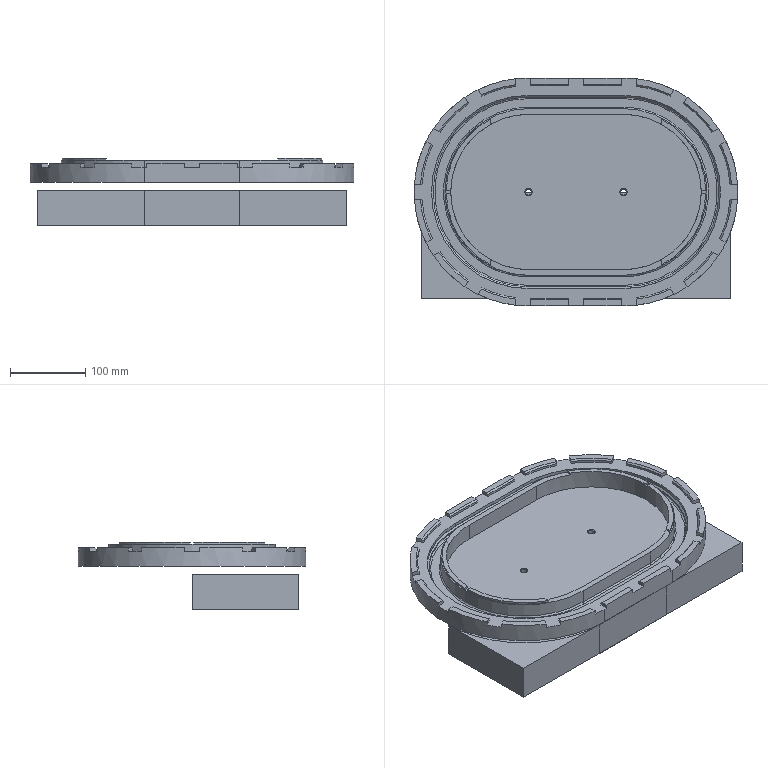NC program | NX | posted with a generic post | part box 429 x 302 x 89.371 mm
Lines 50401 to 52468 of 53366:
(PLANAR_MILL_2 , TOOL : D16开粗)
N100768 T02 M6
N100770 G53
N100772 G17 G0 G90 X220.4 Y-80.6 S6500 M3
N100774 G43 Z50. H2
N100776 Z1.5
N100778 G94 G1 Z-1.5 F3500.
N100780 X204.4
N100782 X189.25
N100784 G2 X179.05 Y-70.408 R10.2
N100786 G3 X63. Y45.55 R116.05
N100788 G1 X-63.
N100790 G3 X-179.05 Y-70.408 R116.05
N100792 G2 X-189.25 Y-80.6 R10.2
N100794 G1 X-204.4
N100796 X-220.4
N100798 Z1.5
N100800 G0 Z50.
N100802 X220.4
N100804 Z0.
N100806 G1 Z-3.
N100808 X204.4
N100810 X189.25
N100812 G2 X179.05 Y-70.408 R10.2
N100814 G3 X63. Y45.55 R116.05
N100816 G1 X-63.
N100818 G3 X-179.05 Y-70.408 R116.05
N100820 G2 X-189.25 Y-80.6 R10.2
N100822 G1 X-204.4
N100824 X-220.4
N100826 Z0.
N100828 G0 Z50.
N100830 X220.4
N100832 Z-1.5
N100834 G1 Z-4.5
N100836 X204.4
N100838 X189.25
N100840 G2 X179.05 Y-70.408 R10.2
N100842 G3 X63. Y45.55 R116.05
N100844 G1 X-63.
N100846 G3 X-179.05 Y-70.408 R116.05
N100848 G2 X-189.25 Y-80.6 R10.2
N100850 G1 X-204.4
N100852 X-220.4
N100854 Z-1.5
N100856 G0 Z50.
N100858 X220.4
N100860 Z-3.
N100862 G1 Z-6.
N100864 X204.4
N100866 X189.25
N100868 G2 X179.05 Y-70.408 R10.2
N100870 G3 X63. Y45.55 R116.05
N100872 G1 X-63.
N100874 G3 X-179.05 Y-70.408 R116.05
N100876 G2 X-189.25 Y-80.6 R10.2
N100878 G1 X-204.4
N100880 X-220.4
N100882 Z-3.
N100884 G0 Z50.
N100886 X220.4
N100888 Z-4.5
N100890 G1 Z-7.5
N100892 X204.4
N100894 X189.25
N100896 G2 X179.05 Y-70.408 R10.2
N100898 G3 X63. Y45.55 R116.05
N100900 G1 X-63.
N100902 G3 X-179.05 Y-70.408 R116.05
N100904 G2 X-189.25 Y-80.6 R10.2
N100906 G1 X-204.4
N100908 X-220.4
N100910 Z-4.5
N100912 G0 Z50.
N100914 X220.4
N100916 Z-6.
N100918 G1 Z-9.
N100920 X204.4
N100922 X189.25
N100924 G2 X179.05 Y-70.408 R10.2
N100926 G3 X63. Y45.55 R116.05
N100928 G1 X-63.
N100930 G3 X-179.05 Y-70.408 R116.05
N100932 G2 X-189.25 Y-80.6 R10.2
N100934 G1 X-204.4
N100936 X-220.4
N100938 Z-6.
N100940 G0 Z50.
N100942 X220.4
N100944 Z-7.5
N100946 G1 Z-10.5
N100948 X204.4
N100950 X189.25
N100952 G2 X179.05 Y-70.408 R10.2
N100954 G3 X63. Y45.55 R116.05
N100956 G1 X-63.
N100958 G3 X-179.05 Y-70.408 R116.05
N100960 G2 X-189.25 Y-80.6 R10.2
N100962 G1 X-204.4
N100964 X-220.4
N100966 Z-7.5
N100968 G0 Z50.
N100970 X220.4
N100972 Z-9.
N100974 G1 Z-12.
N100976 X204.4
N100978 X189.25
N100980 G2 X179.05 Y-70.408 R10.2
N100982 G3 X63. Y45.55 R116.05
N100984 G1 X-63.
N100986 G3 X-179.05 Y-70.408 R116.05
N100988 G2 X-189.25 Y-80.6 R10.2
N100990 G1 X-204.4
N100992 X-220.4
N100994 Z-9.
N100996 G0 Z50.
N100998 X220.4
N101000 Z-10.5
N101002 G1 Z-13.5
N101004 X204.4
N101006 X189.25
N101008 G2 X179.05 Y-70.408 R10.2
N101010 G3 X63. Y45.55 R116.05
N101012 G1 X-63.
N101014 G3 X-179.05 Y-70.408 R116.05
N101016 G2 X-189.25 Y-80.6 R10.2
N101018 G1 X-204.4
N101020 X-220.4
N101022 Z-10.5
N101024 G0 Z50.
N101026 X220.4
N101028 Z-12.
N101030 G1 Z-15.
N101032 X204.4
N101034 X189.25
N101036 G2 X179.05 Y-70.408 R10.2
N101038 G3 X63. Y45.55 R116.05
N101040 G1 X-63.
N101042 G3 X-179.05 Y-70.408 R116.05
N101044 G2 X-189.25 Y-80.6 R10.2
N101046 G1 X-204.4
N101048 X-220.4
N101050 Z-12.
N101052 G0 Z50.
N101054 X220.4
N101056 Z-13.5
N101058 G1 Z-16.5
N101060 X204.4
N101062 X189.25
N101064 G2 X179.05 Y-70.408 R10.2
N101066 G3 X63. Y45.55 R116.05
N101068 G1 X-63.
N101070 G3 X-179.05 Y-70.408 R116.05
N101072 G2 X-189.25 Y-80.6 R10.2
N101074 G1 X-204.4
N101076 X-220.4
N101078 Z-13.5
N101080 G0 Z50.
N101082 X220.4
N101084 Z-15.
N101086 G1 Z-18.
N101088 X204.4
N101090 X189.25
N101092 G2 X179.05 Y-70.408 R10.2
N101094 G3 X63. Y45.55 R116.05
N101096 G1 X-63.
N101098 G3 X-179.05 Y-70.408 R116.05
N101100 G2 X-189.25 Y-80.6 R10.2
N101102 G1 X-204.4
N101104 X-220.4
N101106 Z-15.
N101108 G0 Z50.
N101110 X220.4
N101112 Z-16.5
N101114 G1 Z-19.5
N101116 X204.4
N101118 X189.25
N101120 G2 X179.05 Y-70.408 R10.2
N101122 G3 X63. Y45.55 R116.05
N101124 G1 X-63.
N101126 G3 X-179.05 Y-70.408 R116.05
N101128 G2 X-189.25 Y-80.6 R10.2
N101130 G1 X-204.4
N101132 X-220.4
N101134 Z-16.5
N101136 G0 Z50.
N101138 X220.4
N101140 Z-18.
N101142 G1 Z-21.
N101144 X204.4
N101146 X189.25
N101148 G2 X179.05 Y-70.408 R10.2
N101150 G3 X63. Y45.55 R116.05
N101152 G1 X-63.
N101154 G3 X-179.05 Y-70.408 R116.05
N101156 G2 X-189.25 Y-80.6 R10.2
N101158 G1 X-204.4
N101160 X-220.4
N101162 Z-18.
N101164 G0 Z50.
N101166 X220.4
N101168 Z-19.5
N101170 G1 Z-22.5
N101172 X204.4
N101174 X189.25
N101176 G2 X179.05 Y-70.408 R10.2
N101178 G3 X63. Y45.55 R116.05
N101180 G1 X-63.
N101182 G3 X-179.05 Y-70.408 R116.05
N101184 G2 X-189.25 Y-80.6 R10.2
N101186 G1 X-204.4
N101188 X-220.4
N101190 Z-19.5
N101192 G0 Z50.
N101194 X220.4
N101196 Z-21.
N101198 G1 Z-24.
N101200 X204.4
N101202 X189.25
N101204 G2 X179.05 Y-70.408 R10.2
N101206 G3 X63. Y45.55 R116.05
N101208 G1 X-63.
N101210 G3 X-179.05 Y-70.408 R116.05
N101212 G2 X-189.25 Y-80.6 R10.2
N101214 G1 X-204.4
N101216 X-220.4
N101218 Z-21.
N101220 G0 Z50.
N101222 X220.4
N101224 Z-22.5
N101226 G1 Z-25.5
N101228 X204.4
N101230 X189.25
N101232 G2 X179.05 Y-70.408 R10.2
N101234 G3 X63. Y45.55 R116.05
N101236 G1 X-63.
N101238 G3 X-179.05 Y-70.408 R116.05
N101240 G2 X-189.25 Y-80.6 R10.2
N101242 G1 X-204.4
N101244 X-220.4
N101246 Z-22.5
N101248 G0 Z50.
N101250 X220.4
N101252 Z-24.
N101254 G1 Z-27.
N101256 X204.4
N101258 X189.25
N101260 G2 X179.05 Y-70.408 R10.2
N101262 G3 X63. Y45.55 R116.05
N101264 G1 X-63.
N101266 G3 X-179.05 Y-70.408 R116.05
N101268 G2 X-189.25 Y-80.6 R10.2
N101270 G1 X-204.4
N101272 X-220.4
N101274 Z-24.
N101276 G0 Z50.
N101278 X220.4
N101280 Z-25.5
N101282 G1 Z-28.5
N101284 X204.4
N101286 X189.25
N101288 G2 X179.05 Y-70.408 R10.2
N101290 G3 X63. Y45.55 R116.05
N101292 G1 X-63.
N101294 G3 X-179.05 Y-70.408 R116.05
N101296 G2 X-189.25 Y-80.6 R10.2
N101298 G1 X-204.4
N101300 X-220.4
N101302 Z-25.5
N101304 G0 Z50.
N101306 X220.4
N101308 Z-27.
N101310 G1 Z-30.
N101312 X204.4
N101314 X189.25
N101316 G2 X179.05 Y-70.408 R10.2
N101318 G3 X63. Y45.55 R116.05
N101320 G1 X-63.
N101322 G3 X-179.05 Y-70.408 R116.05
N101324 G2 X-189.25 Y-80.6 R10.2
N101326 G1 X-204.4
N101328 X-220.4
N101330 Z-27.
N101332 G0 Z50.
N101334 X220.4
N101336 Z-28.5
N101338 G1 Z-31.5
N101340 X204.4
N101342 X189.25
N101344 G2 X179.05 Y-70.408 R10.2
N101346 G3 X63. Y45.55 R116.05
N101348 G1 X-63.
N101350 G3 X-179.05 Y-70.408 R116.05
N101352 G2 X-189.25 Y-80.6 R10.2
N101354 G1 X-204.4
N101356 X-220.4
N101358 Z-28.5
N101360 G0 Z50.
N101362 X220.4
N101364 Z-30.
N101366 G1 Z-33.
N101368 X204.4
N101370 X189.25
N101372 G2 X179.05 Y-70.408 R10.2
N101374 G3 X63. Y45.55 R116.05
N101376 G1 X-63.
N101378 G3 X-179.05 Y-70.408 R116.05
N101380 G2 X-189.25 Y-80.6 R10.2
N101382 G1 X-204.4
N101384 X-220.4
N101386 Z-30.
N101388 G0 Z50.
N101390 X220.4
N101392 Z-31.5
N101394 G1 Z-34.5
N101396 X204.4
N101398 X189.25
N101400 G2 X179.05 Y-70.408 R10.2
N101402 G3 X63. Y45.55 R116.05
N101404 G1 X-63.
N101406 G3 X-179.05 Y-70.408 R116.05
N101408 G2 X-189.25 Y-80.6 R10.2
N101410 G1 X-204.4
N101412 X-220.4
N101414 Z-31.5
N101416 G0 Z50.
N101418 X220.4
N101420 Z-33.
N101422 G1 Z-36.
N101424 X204.4
N101426 X189.25
N101428 G2 X179.05 Y-70.408 R10.2
N101430 G3 X63. Y45.55 R116.05
N101432 G1 X-63.
N101434 G3 X-179.05 Y-70.408 R116.05
N101436 G2 X-189.25 Y-80.6 R10.2
N101438 G1 X-204.4
N101440 X-220.4
N101442 Z-33.
N101444 G0 Z50.
N101446 X220.4
N101448 Z-34.5
N101450 G1 Z-37.5
N101452 X204.4
N101454 X189.25
N101456 G2 X179.05 Y-70.408 R10.2
N101458 G3 X63. Y45.55 R116.05
N101460 G1 X-63.
N101462 G3 X-179.05 Y-70.408 R116.05
N101464 G2 X-189.25 Y-80.6 R10.2
N101466 G1 X-204.4
N101468 X-220.4
N101470 Z-34.5
N101472 G0 Z50.
N101474 X220.4
N101476 Z-36.
N101478 G1 Z-39.
N101480 X204.4
N101482 X189.25
N101484 G2 X179.05 Y-70.408 R10.2
N101486 G3 X63. Y45.55 R116.05
N101488 G1 X-63.
N101490 G3 X-179.05 Y-70.408 R116.05
N101492 G2 X-189.25 Y-80.6 R10.2
N101494 G1 X-204.4
N101496 X-220.4
N101498 Z-36.
N101500 G0 Z50.
N101502 X220.4
N101504 Z-37.5
N101506 G1 Z-40.5
N101508 X204.4
N101510 X189.25
N101512 G2 X179.05 Y-70.408 R10.2
N101514 G3 X63. Y45.55 R116.05
N101516 G1 X-63.
N101518 G3 X-179.05 Y-70.408 R116.05
N101520 G2 X-189.25 Y-80.6 R10.2
N101522 G1 X-204.4
N101524 X-220.4
N101526 Z-37.5
N101528 G0 Z50.
N101530 X220.4
N101532 Z-39.
N101534 G1 Z-42.
N101536 X204.4
N101538 X189.25
N101540 G2 X179.05 Y-70.408 R10.2
N101542 G3 X63. Y45.55 R116.05
N101544 G1 X-63.
N101546 G3 X-179.05 Y-70.408 R116.05
N101548 G2 X-189.25 Y-80.6 R10.2
N101550 G1 X-204.4
N101552 X-220.4
N101554 Z-39.
N101556 G0 Z50.
N101558 X220.4
N101560 Z-40.5
N101562 G1 Z-43.5
N101564 X204.4
N101566 X189.25
N101568 G2 X179.05 Y-70.408 R10.2
N101570 G3 X63. Y45.55 R116.05
N101572 G1 X-63.
N101574 G3 X-179.05 Y-70.408 R116.05
N101576 G2 X-189.25 Y-80.6 R10.2
N101578 G1 X-204.4
N101580 X-220.4
N101582 Z-40.5
N101584 G0 Z50.
N101586 X220.4
N101588 Z-42.
N101590 G1 Z-45.
N101592 X204.4
N101594 X189.25
N101596 G2 X179.05 Y-70.408 R10.2
N101598 G3 X63. Y45.55 R116.05
N101600 G1 X-63.
N101602 G3 X-179.05 Y-70.408 R116.05
N101604 G2 X-189.25 Y-80.6 R10.2
N101606 G1 X-204.4
N101608 X-220.4
N101610 Z-42.
N101612 G0 Z50.
N101614 X220.4
N101616 Z-43.5
N101618 G1 Z-46.5
N101620 X204.4
N101622 X189.25
N101624 G2 X179.05 Y-70.408 R10.2
N101626 G3 X63. Y45.55 R116.05
N101628 G1 X-63.
N101630 G3 X-179.05 Y-70.408 R116.05
N101632 G2 X-189.25 Y-80.6 R10.2
N101634 G1 X-204.4
N101636 X-220.4
N101638 Z-43.5
N101640 G0 Z50.
N101642 X220.4
N101644 Z-45.
N101646 G1 Z-48.
N101648 X204.4
N101650 X189.25
N101652 G2 X179.05 Y-70.408 R10.2
N101654 G3 X63. Y45.55 R116.05
N101656 G1 X-63.
N101658 G3 X-179.05 Y-70.408 R116.05
N101660 G2 X-189.25 Y-80.6 R10.2
N101662 G1 X-204.4
N101664 X-220.4
N101666 Z-45.
N101668 G0 Z50.
N101670 X220.4
N101672 Z-46.5
N101674 G1 Z-49.5
N101676 X204.4
N101678 X189.25
N101680 G2 X179.05 Y-70.408 R10.2
N101682 G3 X63. Y45.55 R116.05
N101684 G1 X-63.
N101686 G3 X-179.05 Y-70.408 R116.05
N101688 G2 X-189.25 Y-80.6 R10.2
N101690 G1 X-204.4
N101692 X-220.4
N101694 Z-46.5
N101696 G0 Z50.
N101698 X220.4
N101700 Z-46.8
N101702 G1 Z-49.8
N101704 X204.4
N101706 X189.25
N101708 G2 X179.05 Y-70.408 R10.2
N101710 G3 X63. Y45.55 R116.05
N101712 G1 X-63.
N101714 G3 X-179.05 Y-70.408 R116.05
N101716 G2 X-189.25 Y-80.6 R10.2
N101718 G1 X-204.4
N101720 X-220.4
N101722 Z-46.8
N101724 G0 Z50.
(PLANAR_MILL_2_COPY_2 , TOOL : D16开粗)
N101726 X184.207 Y-79.408
N101728 Z2.
N101730 G1 Z-1. F3000.
N101732 X184.2 Y-70.408
N101734 G3 X63.5 Y50.2 R120.7
N101736 G1 X-63.5
N101738 G3 X-184.2 Y-70.408 R120.7
N101740 G1 X-184.207 Y-79.408
N101742 Z2.
N101744 G0 Z50.
N101746 X184.207
N101748 Z1.
N101750 G1 Z-2.
N101752 X184.2 Y-70.408
N101754 G3 X63.5 Y50.2 R120.7
N101756 G1 X-63.5
N101758 G3 X-184.2 Y-70.408 R120.7
N101760 G1 X-184.207 Y-79.408
N101762 Z1.
N101764 G0 Z50.
N101766 X184.207
N101768 Z0.
N101770 G1 Z-3.
N101772 X184.2 Y-70.408
N101774 G3 X63.5 Y50.2 R120.7
N101776 G1 X-63.5
N101778 G3 X-184.2 Y-70.408 R120.7
N101780 G1 X-184.207 Y-79.408
N101782 Z0.
N101784 G0 Z50.
N101786 X184.207
N101788 Z-1.
N101790 G1 Z-4.
N101792 X184.2 Y-70.408
N101794 G3 X63.5 Y50.2 R120.7
N101796 G1 X-63.5
N101798 G3 X-184.2 Y-70.408 R120.7
N101800 G1 X-184.207 Y-79.408
N101802 Z-1.
N101804 G0 Z50.
N101806 X184.207
N101808 Z-2.
N101810 G1 Z-5.
N101812 X184.2 Y-70.408
N101814 G3 X63.5 Y50.2 R120.7
N101816 G1 X-63.5
N101818 G3 X-184.2 Y-70.408 R120.7
N101820 G1 X-184.207 Y-79.408
N101822 Z-2.
N101824 G0 Z50.
N101826 X184.207
N101828 Z-3.
N101830 G1 Z-6.
N101832 X184.2 Y-70.408
N101834 G3 X63.5 Y50.2 R120.7
N101836 G1 X-63.5
N101838 G3 X-184.2 Y-70.408 R120.7
N101840 G1 X-184.207 Y-79.408
N101842 Z-3.
N101844 G0 Z50.
N101846 X184.207
N101848 Z-4.
N101850 G1 Z-7.
N101852 X184.2 Y-70.408
N101854 G3 X63.5 Y50.2 R120.7
N101856 G1 X-63.5
N101858 G3 X-184.2 Y-70.408 R120.7
N101860 G1 X-184.207 Y-79.408
N101862 Z-4.
N101864 G0 Z50.
N101866 X184.207
N101868 Z-5.
N101870 G1 Z-8.
N101872 X184.2 Y-70.408
N101874 G3 X63.5 Y50.2 R120.7
N101876 G1 X-63.5
N101878 G3 X-184.2 Y-70.408 R120.7
N101880 G1 X-184.207 Y-79.408
N101882 Z-5.
N101884 G0 Z50.
N101886 X184.207
N101888 Z-6.
N101890 G1 Z-9.
N101892 X184.2 Y-70.408
N101894 G3 X63.5 Y50.2 R120.7
N101896 G1 X-63.5
N101898 G3 X-184.2 Y-70.408 R120.7
N101900 G1 X-184.207 Y-79.408
N101902 Z-6.
N101904 G0 Z50.
N101906 X184.207
N101908 Z-7.
N101910 G1 Z-10.
N101912 X184.2 Y-70.408
N101914 G3 X63.5 Y50.2 R120.7
N101916 G1 X-63.5
N101918 G3 X-184.2 Y-70.408 R120.7
N101920 G1 X-184.207 Y-79.408
N101922 Z-7.
N101924 G0 Z50.
N101926 X184.207
N101928 Z-8.
N101930 G1 Z-11.
N101932 X184.2 Y-70.408
N101934 G3 X63.5 Y50.2 R120.7
N101936 G1 X-63.5
N101938 G3 X-184.2 Y-70.408 R120.7
N101940 G1 X-184.207 Y-79.408
N101942 Z-8.
N101944 G0 Z50.
N101946 X184.207
N101948 Z-9.
N101950 G1 Z-12.
N101952 X184.2 Y-70.408
N101954 G3 X63.5 Y50.2 R120.7
N101956 G1 X-63.5
N101958 G3 X-184.2 Y-70.408 R120.7
N101960 G1 X-184.207 Y-79.408
N101962 Z-9.
N101964 G0 Z50.
N101966 X184.207
N101968 Z-10.
N101970 G1 Z-13.
N101972 X184.2 Y-70.408
N101974 G3 X63.5 Y50.2 R120.7
N101976 G1 X-63.5
N101978 G3 X-184.2 Y-70.408 R120.7
N101980 G1 X-184.207 Y-79.408
N101982 Z-10.
N101984 G0 Z50.
N101986 X184.207
N101988 Z-11.
N101990 G1 Z-14.
N101992 X184.2 Y-70.408
N101994 G3 X63.5 Y50.2 R120.7
N101996 G1 X-63.5
N101998 G3 X-184.2 Y-70.408 R120.7
N102000 G1 X-184.207 Y-79.408
N102002 Z-11.
N102004 G0 Z50.
N102006 X184.207
N102008 Z-12.
N102010 G1 Z-15.
N102012 X184.2 Y-70.408
N102014 G3 X63.5 Y50.2 R120.7
N102016 G1 X-63.5
N102018 G3 X-184.2 Y-70.408 R120.7
N102020 G1 X-184.207 Y-79.408
N102022 Z-12.
N102024 G0 Z50.
N102026 X184.207
N102028 Z-13.
N102030 G1 Z-16.
N102032 X184.2 Y-70.408
N102034 G3 X63.5 Y50.2 R120.7
N102036 G1 X-63.5
N102038 G3 X-184.2 Y-70.408 R120.7
N102040 G1 X-184.207 Y-79.408
N102042 Z-13.
N102044 G0 Z50.
N102046 X184.207
N102048 Z-14.
N102050 G1 Z-17.
N102052 X184.2 Y-70.408
N102054 G3 X63.5 Y50.2 R120.7
N102056 G1 X-63.5
N102058 G3 X-184.2 Y-70.408 R120.7
N102060 G1 X-184.207 Y-79.408
N102062 Z-14.
N102064 G0 Z50.
N102066 X184.207
N102068 Z-15.
N102070 G1 Z-18.
N102072 X184.2 Y-70.408
N102074 G3 X63.5 Y50.2 R120.7
N102076 G1 X-63.5
N102078 G3 X-184.2 Y-70.408 R120.7
N102080 G1 X-184.207 Y-79.408
N102082 Z-15.
N102084 G0 Z50.
N102086 X184.207
N102088 Z-16.
N102090 G1 Z-19.
N102092 X184.2 Y-70.408
N102094 G3 X63.5 Y50.2 R120.7
N102096 G1 X-63.5
N102098 G3 X-184.2 Y-70.408 R120.7
N102100 G1 X-184.207 Y-79.408
N102102 Z-16.
N102104 G0 Z50.
N102106 X184.207
N102108 Z-17.
N102110 G1 Z-20.
N102112 X184.2 Y-70.408
N102114 G3 X63.5 Y50.2 R120.7
N102116 G1 X-63.5
N102118 G3 X-184.2 Y-70.408 R120.7
N102120 G1 X-184.207 Y-79.408
N102122 Z-17.
N102124 G0 Z50.
N102126 X184.207
N102128 Z-18.
N102130 G1 Z-21.
N102132 X184.2 Y-70.408
N102134 G3 X63.5 Y50.2 R120.7
N102136 G1 X-63.5
N102138 G3 X-184.2 Y-70.408 R120.7
N102140 G1 X-184.207 Y-79.408
N102142 Z-18.
N102144 G0 Z50.
N102146 X184.207
N102148 Z-19.
N102150 G1 Z-22.
N102152 X184.2 Y-70.408
N102154 G3 X63.5 Y50.2 R120.7
N102156 G1 X-63.5
N102158 G3 X-184.2 Y-70.408 R120.7
N102160 G1 X-184.207 Y-79.408
N102162 Z-19.
N102164 G0 Z50.
N102166 X184.207
N102168 Z-20.
N102170 G1 Z-23.
N102172 X184.2 Y-70.408
N102174 G3 X63.5 Y50.2 R120.7
N102176 G1 X-63.5
N102178 G3 X-184.2 Y-70.408 R120.7
N102180 G1 X-184.207 Y-79.408
N102182 Z-20.
N102184 G0 Z50.
N102186 X184.207
N102188 Z-20.886
N102190 G1 Z-23.886
N102192 X184.2 Y-70.408
N102194 G3 X63.5 Y50.2 R120.7
N102196 G1 X-63.5
N102198 G3 X-184.2 Y-70.408 R120.7
N102200 G1 X-184.207 Y-79.408
N102202 Z-20.886
N102204 G0 Z50.
(PLANAR_MILL_2_COPY_2_COPY , TOOL : D16开粗)
N102206 X184.312 Y-86.408
N102208 Z-20.886
N102210 G1 Z-23.886 F800.
N102212 X184.3 Y-70.408
N102214 G3 X63.5 Y50.3 R120.8
N102216 G1 X-63.5
N102218 G3 X-184.3 Y-70.408 R120.8
N102220 G1 X-184.312 Y-86.408
N102222 Z-20.886
N102224 G0 Z50.
(PLANAR_MILL_2_COPY_1 , TOOL : D16开粗)
N102226 X220.4 Y-80.5
N102228 Z-46.95
N102230 G1 Z-49.95
N102232 X204.4
N102234 X189.25
N102236 G2 X179.15 Y-70.408 R10.1
N102238 G3 X63. Y45.65 R116.15
N102240 G1 X-63.
N102242 G3 X-179.15 Y-70.408 R116.15
N102244 G2 X-189.25 Y-80.5 R10.1
N102246 G1 X-204.4
N102248 X-220.4
N102250 Z-46.95
N102252 G0 Z50.
N102254 M5
(FLOOR_FACING , TOOL : D63.)
N102256 T01 M6
N102258 G54
N102260 G17 G0 G90 X160.741 Y104.9 S4500 M3
N102262 G43 Z50. H1
N102264 Z3.
N102266 G94 G1 Z0. F1500.
N102268 Y101.9
N102270 Y-101.9
N102272 Y-104.9
N102274 Z3.
N102276 G0 Z50.
N102278 X116.236 Y104.9
N102280 Z3.
N102282 G1 Z0.
N102284 Y101.9
N102286 Y-101.9
N102288 Y-104.9
N102290 Z3.
N102292 G0 Z50.
N102294 X71.731 Y104.9
N102296 Z3.
N102298 G1 Z0.
N102300 Y101.9
N102302 Y-101.9
N102304 Y-104.9
N102306 Z3.
N102308 G0 Z50.
N102310 X27.226 Y104.9
N102312 Z3.
N102314 G1 Z0.
N102316 Y101.9
N102318 Y-101.9
N102320 Y-104.9
N102322 Z3.
N102324 G0 Z50.
N102326 X-17.279 Y104.9
N102328 Z3.
N102330 G1 Z0.
N102332 Y101.9
N102334 Y-101.9
N102336 Y-104.9
N102338 Z3.
N102340 G0 Z50.
N102342 X-61.784 Y104.9
N102344 Z3.
N102346 G1 Z0.
N102348 Y101.9
N102350 Y-101.9
N102352 Y-104.9
N102354 Z3.
N102356 G0 Z50.
N102358 X-106.289 Y104.9
N102360 Z3.
N102362 G1 Z0.
N102364 Y101.9
N102366 Y-101.9
N102368 Y-104.9
N102370 Z3.
N102372 G0 Z50.
N102374 X-150.794 Y127.755
N102376 Z3.
N102378 G1 Z0.
N102380 Y101.9
N102382 Y-101.9
N102384 Y-118.902
N102386 Z3.
N102388 G0 Z50.
N102390 M5
(DRILLING_COPY , TOOL : 倒角12.)
N102392 T03 M6
N102394 G54
N102396 G17 G0 G90 X-154.4 Y-30.4 S1500 M3
N102398 G43 Z50. H3
N102400 G94 G81 G98 Z-5.5 F150. R3.
N102402 X-74.4 Y29.6
N102404 X74.4
N102406 X154.4 Y-30.4
N102408 G80
N102410 G0 X154.4 Y-30.4 Z50.
N102412 M5
(DRILLING , TOOL : 钻头10.5)
N102414 T04 M6
N102416 G54
N102418 G17 G0 G90 X-154.4 Y-30.4 S1200 M3
N102420 G43 Z50. H4
N102422 G94 G83 G98 Z-57. F180. Q5. R3.
N102424 X-74.4 Y29.6
N102426 X74.4
N102428 X154.4 Y-30.4
N102430 G80
N102432 G0 X154.4 Y-30.4 Z50.
N102434 M5
(DRILLING_COPY_1 , TOOL : D16开粗)
N102436 T02 M6
N102438 G54
N102440 G17 G0 G90 X-154.4 Y-30.4 S700 M3
N102442 G43 Z50. H2
N102444 G94 G83 G98 Z-15. F120. Q2. R3.
N102446 X-74.4 Y29.6
N102448 X74.4
N102450 X154.4 Y-30.4
N102452 G80
N102454 G0 X154.4 Y-30.4 Z50.
N102456 M5
(PLANAR_MILL_COPY_1 , TOOL : D63.)
N102458 T01 M6
N102460 G54
N102462 G17 G0 G90 X-190.948 Y-63.003 S4500 M3
N102464 G43 Z50. H1
N102466 Z3.1
N102468 G94 G1 Z0.1 F1500.
N102470 X-190.9 Y-0.003
N102472 G2 X-63.5 Y127.3 R127.4
N102474 G1 X63.5
N102476 G2 X190.9 Y-0.003 R127.4
N102478 G1 X190.948 Y-63.003
N102480 Z3.1
N102482 G0 Z50.
N102484 M5
(PLANAR_MILL_2_COPY_2_COPY_1 , TOOL : D16开粗)
N102486 T02 M6
N102488 G54
N102490 G17 G0 G90 X213.4 Y-8.1 S6500 M3
N102492 G43 Z50. H2
N102494 Z1.5
N102496 G94 G1 Z-1.5 F3000.
N102498 X204.4
N102500 X194.4
N102502 G2 X186.3 Y-0.006 R8.1
N102504 G3 X63.5 Y122.7 R122.8
N102506 G1 X-63.5
N102508 G3 X-186.3 Y-0.006 R122.8
N102510 G2 X-194.4 Y-8.1 R8.1
N102512 G1 X-204.4
N102514 X-213.4
N102516 Z1.5
N102518 G0 Z3.
N102520 X213.4
N102522 Z0.
N102524 G1 Z-3.
N102526 X204.4
N102528 X194.4
N102530 G2 X186.3 Y-0.006 R8.1
N102532 G3 X63.5 Y122.7 R122.8
N102534 G1 X-63.5
N102536 G3 X-186.3 Y-0.006 R122.8
N102538 G2 X-194.4 Y-8.1 R8.1
N102540 G1 X-204.4
N102542 X-213.4
N102544 Z0.
N102546 G0 Z3.
N102548 X213.4
N102550 Z-1.5
N102552 G1 Z-4.5
N102554 X204.4
N102556 X194.4
N102558 G2 X186.3 Y-0.006 R8.1
N102560 G3 X63.5 Y122.7 R122.8
N102562 G1 X-63.5
N102564 G3 X-186.3 Y-0.006 R122.8
N102566 G2 X-194.4 Y-8.1 R8.1
N102568 G1 X-204.4
N102570 X-213.4
N102572 Z-1.5
N102574 G0 Z3.
N102576 X213.4
N102578 Z-3.
N102580 G1 Z-6.
N102582 X204.4
N102584 X194.4
N102586 G2 X186.3 Y-0.006 R8.1
N102588 G3 X63.5 Y122.7 R122.8
N102590 G1 X-63.5
N102592 G3 X-186.3 Y-0.006 R122.8
N102594 G2 X-194.4 Y-8.1 R8.1
N102596 G1 X-204.4
N102598 X-213.4
N102600 Z-3.
N102602 G0 Z3.
N102604 X213.4
N102606 Z-4.5
N102608 G1 Z-7.5
N102610 X204.4
N102612 X194.4
N102614 G2 X186.3 Y-0.006 R8.1
N102616 G3 X63.5 Y122.7 R122.8
N102618 G1 X-63.5
N102620 G3 X-186.3 Y-0.006 R122.8
N102622 G2 X-194.4 Y-8.1 R8.1
N102624 G1 X-204.4
N102626 X-213.4
N102628 Z-4.5
N102630 G0 Z3.
N102632 X213.4
N102634 Z-6.
N102636 G1 Z-9.
N102638 X204.4
N102640 X194.4
N102642 G2 X186.3 Y-0.006 R8.1
N102644 G3 X63.5 Y122.7 R122.8
N102646 G1 X-63.5
N102648 G3 X-186.3 Y-0.006 R122.8
N102650 G2 X-194.4 Y-8.1 R8.1
N102652 G1 X-204.4
N102654 X-213.4
N102656 Z-6.
N102658 G0 Z3.
N102660 X213.4
N102662 Z-7.5
N102664 G1 Z-10.5
N102666 X204.4
N102668 X194.4
N102670 G2 X186.3 Y-0.006 R8.1
N102672 G3 X63.5 Y122.7 R122.8
N102674 G1 X-63.5
N102676 G3 X-186.3 Y-0.006 R122.8
N102678 G2 X-194.4 Y-8.1 R8.1
N102680 G1 X-204.4
N102682 X-213.4
N102684 Z-7.5
N102686 G0 Z3.
N102688 X213.4
N102690 Z-9.
N102692 G1 Z-12.
N102694 X204.4
N102696 X194.4
N102698 G2 X186.3 Y-0.006 R8.1
N102700 G3 X63.5 Y122.7 R122.8
N102702 G1 X-63.5
N102704 G3 X-186.3 Y-0.006 R122.8
N102706 G2 X-194.4 Y-8.1 R8.1
N102708 G1 X-204.4
N102710 X-213.4
N102712 Z-9.
N102714 G0 Z3.
N102716 X213.4
N102718 Z-10.5
N102720 G1 Z-13.5
N102722 X204.4
N102724 X194.4
N102726 G2 X186.3 Y-0.006 R8.1
N102728 G3 X63.5 Y122.7 R122.8
N102730 G1 X-63.5
N102732 G3 X-186.3 Y-0.006 R122.8
N102734 G2 X-194.4 Y-8.1 R8.1
N102736 G1 X-204.4
N102738 X-213.4
N102740 Z-10.5
N102742 G0 Z3.
N102744 X213.4
N102746 Z-12.
N102748 G1 Z-15.
N102750 X204.4
N102752 X194.4
N102754 G2 X186.3 Y-0.006 R8.1
N102756 G3 X63.5 Y122.7 R122.8
N102758 G1 X-63.5
N102760 G3 X-186.3 Y-0.006 R122.8
N102762 G2 X-194.4 Y-8.1 R8.1
N102764 G1 X-204.4
N102766 X-213.4
N102768 Z-12.
N102770 G0 Z3.
N102772 X213.4
N102774 Z-13.5
N102776 G1 Z-16.5
N102778 X204.4
N102780 X194.4
N102782 G2 X186.3 Y-0.006 R8.1
N102784 G3 X63.5 Y122.7 R122.8
N102786 G1 X-63.5
N102788 G3 X-186.3 Y-0.006 R122.8
N102790 G2 X-194.4 Y-8.1 R8.1
N102792 G1 X-204.4
N102794 X-213.4
N102796 Z-13.5
N102798 G0 Z3.
N102800 X213.4
N102802 Z-15.
N102804 G1 Z-18.
N102806 X204.4
N102808 X194.4
N102810 G2 X186.3 Y-0.006 R8.1
N102812 G3 X63.5 Y122.7 R122.8
N102814 G1 X-63.5
N102816 G3 X-186.3 Y-0.006 R122.8
N102818 G2 X-194.4 Y-8.1 R8.1
N102820 G1 X-204.4
N102822 X-213.4
N102824 Z-15.
N102826 G0 Z3.
N102828 X213.4
N102830 Z-16.5
N102832 G1 Z-19.5
N102834 X204.4
N102836 X194.4
N102838 G2 X186.3 Y-0.006 R8.1
N102840 G3 X63.5 Y122.7 R122.8
N102842 G1 X-63.5
N102844 G3 X-186.3 Y-0.006 R122.8
N102846 G2 X-194.4 Y-8.1 R8.1
N102848 G1 X-204.4
N102850 X-213.4
N102852 Z-16.5
N102854 G0 Z3.
N102856 X213.4
N102858 Z-18.
N102860 G1 Z-21.
N102862 X204.4
N102864 X194.4
N102866 G2 X186.3 Y-0.006 R8.1
N102868 G3 X63.5 Y122.7 R122.8
N102870 G1 X-63.5
N102872 G3 X-186.3 Y-0.006 R122.8
N102874 G2 X-194.4 Y-8.1 R8.1
N102876 G1 X-204.4
N102878 X-213.4
N102880 Z-18.
N102882 G0 Z3.
N102884 X213.4
N102886 Z-19.5
N102888 G1 Z-22.5
N102890 X204.4
N102892 X194.4
N102894 G2 X186.3 Y-0.006 R8.1
N102896 G3 X63.5 Y122.7 R122.8
N102898 G1 X-63.5
N102900 G3 X-186.3 Y-0.006 R122.8
N102902 G2 X-194.4 Y-8.1 R8.1
N102904 G1 X-204.4
N102906 X-213.4
N102908 Z-19.5
N102910 G0 Z3.
N102912 X213.4
N102914 Z-21.
N102916 G1 Z-24.
N102918 X204.4
N102920 X194.4
N102922 G2 X186.3 Y-0.006 R8.1
N102924 G3 X63.5 Y122.7 R122.8
N102926 G1 X-63.5
N102928 G3 X-186.3 Y-0.006 R122.8
N102930 G2 X-194.4 Y-8.1 R8.1
N102932 G1 X-204.4
N102934 X-213.4
N102936 Z-21.
N102938 G0 Z3.
N102940 X213.4
N102942 Z-22.5
N102944 G1 Z-25.5
N102946 X204.4
N102948 X194.4
N102950 G2 X186.3 Y-0.006 R8.1
N102952 G3 X63.5 Y122.7 R122.8
N102954 G1 X-63.5
N102956 G3 X-186.3 Y-0.006 R122.8
N102958 G2 X-194.4 Y-8.1 R8.1
N102960 G1 X-204.4
N102962 X-213.4
N102964 Z-22.5
N102966 G0 Z3.
N102968 X213.4
N102970 Z-22.786
N102972 G1 Z-25.786
N102974 X204.4
N102976 X194.4
N102978 G2 X186.3 Y-0.006 R8.1
N102980 G3 X63.5 Y122.7 R122.8
N102982 G1 X-63.5
N102984 G3 X-186.3 Y-0.006 R122.8
N102986 G2 X-194.4 Y-8.1 R8.1
N102988 G1 X-204.4
N102990 X-213.4
N102992 Z-22.786
N102994 G0 Z50.
(PLANAR_MILL_2_COPY_3 , TOOL : D16开粗)
N102996 X220.4
N102998 Z-21.886
N103000 G1 Z-24.886 F3500.
N103002 X204.4
N103004 X189.25
N103006 G2 X181.15 Y-0.006 R8.1
N103008 G3 X63. Y118.05 R118.15
N103010 G1 X-63.
N103012 G3 X-181.15 Y-0.006 R118.15
N103014 G2 X-189.25 Y-8.1 R8.1
N103016 G1 X-204.4
N103018 X-220.4
N103020 Z-21.886
N103022 G0 Z50.
N103024 X220.4
N103026 Z-23.386
N103028 G1 Z-26.386
N103030 X204.4
N103032 X189.25
N103034 G2 X181.15 Y-0.006 R8.1
N103036 G3 X63. Y118.05 R118.15
N103038 G1 X-63.
N103040 G3 X-181.15 Y-0.006 R118.15
N103042 G2 X-189.25 Y-8.1 R8.1
N103044 G1 X-204.4
N103046 X-220.4
N103048 Z-23.386
N103050 G0 Z50.
N103052 X220.4
N103054 Z-24.886
N103056 G1 Z-27.886
N103058 X204.4
N103060 X189.25
N103062 G2 X181.15 Y-0.006 R8.1
N103064 G3 X63. Y118.05 R118.15
N103066 G1 X-63.
N103068 G3 X-181.15 Y-0.006 R118.15
N103070 G2 X-189.25 Y-8.1 R8.1
N103072 G1 X-204.4
N103074 X-220.4
N103076 Z-24.886
N103078 G0 Z50.
N103080 X220.4
N103082 Z-26.386
N103084 G1 Z-29.386
N103086 X204.4
N103088 X189.25
N103090 G2 X181.15 Y-0.006 R8.1
N103092 G3 X63. Y118.05 R118.15
N103094 G1 X-63.
N103096 G3 X-181.15 Y-0.006 R118.15
N103098 G2 X-189.25 Y-8.1 R8.1
N103100 G1 X-204.4
N103102 X-220.4
N103104 Z-26.386
N103106 G0 Z50.
N103108 X220.4
N103110 Z-27.886
N103112 G1 Z-30.886
N103114 X204.4
N103116 X189.25
N103118 G2 X181.15 Y-0.006 R8.1
N103120 G3 X63. Y118.05 R118.15
N103122 G1 X-63.
N103124 G3 X-181.15 Y-0.006 R118.15
N103126 G2 X-189.25 Y-8.1 R8.1
N103128 G1 X-204.4
N103130 X-220.4
N103132 Z-27.886
N103134 G0 Z50.
N103136 X220.4
N103138 Z-29.386
N103140 G1 Z-32.386
N103142 X204.4
N103144 X189.25
N103146 G2 X181.15 Y-0.006 R8.1
N103148 G3 X63. Y118.05 R118.15
N103150 G1 X-63.
N103152 G3 X-181.15 Y-0.006 R118.15
N103154 G2 X-189.25 Y-8.1 R8.1
N103156 G1 X-204.4
N103158 X-220.4
N103160 Z-29.386
N103162 G0 Z50.
N103164 X220.4
N103166 Z-30.886
N103168 G1 Z-33.886
N103170 X204.4
N103172 X189.25
N103174 G2 X181.15 Y-0.006 R8.1
N103176 G3 X63. Y118.05 R118.15
N103178 G1 X-63.
N103180 G3 X-181.15 Y-0.006 R118.15
N103182 G2 X-189.25 Y-8.1 R8.1
N103184 G1 X-204.4
N103186 X-220.4
N103188 Z-30.886
N103190 G0 Z50.
N103192 X220.4
N103194 Z-32.386
N103196 G1 Z-35.386
N103198 X204.4
N103200 X189.25
N103202 G2 X181.15 Y-0.006 R8.1
N103204 G3 X63. Y118.05 R118.15
N103206 G1 X-63.
N103208 G3 X-181.15 Y-0.006 R118.15
N103210 G2 X-189.25 Y-8.1 R8.1
N103212 G1 X-204.4
N103214 X-220.4
N103216 Z-32.386
N103218 G0 Z50.
N103220 X220.4
N103222 Z-33.886
N103224 G1 Z-36.886
N103226 X204.4
N103228 X189.25
N103230 G2 X181.15 Y-0.006 R8.1
N103232 G3 X63. Y118.05 R118.15
N103234 G1 X-63.
N103236 G3 X-181.15 Y-0.006 R118.15
N103238 G2 X-189.25 Y-8.1 R8.1
N103240 G1 X-204.4
N103242 X-220.4
N103244 Z-33.886
N103246 G0 Z50.
N103248 X220.4
N103250 Z-35.386
N103252 G1 Z-38.386
N103254 X204.4
N103256 X189.25
N103258 G2 X181.15 Y-0.006 R8.1
N103260 G3 X63. Y118.05 R118.15
N103262 G1 X-63.
N103264 G3 X-181.15 Y-0.006 R118.15
N103266 G2 X-189.25 Y-8.1 R8.1
N103268 G1 X-204.4
N103270 X-220.4
N103272 Z-35.386
N103274 G0 Z50.
N103276 X220.4
N103278 Z-36.886
N103280 G1 Z-39.886
N103282 X204.4
N103284 X189.25
N103286 G2 X181.15 Y-0.006 R8.1
N103288 G3 X63. Y118.05 R118.15
N103290 G1 X-63.
N103292 G3 X-181.15 Y-0.006 R118.15
N103294 G2 X-189.25 Y-8.1 R8.1
N103296 G1 X-204.4
N103298 X-220.4
N103300 Z-36.886
N103302 G0 Z50.
N103304 X220.4
N103306 Z-38.386
N103308 G1 Z-41.386
N103310 X204.4
N103312 X189.25
N103314 G2 X181.15 Y-0.006 R8.1
N103316 G3 X63. Y118.05 R118.15
N103318 G1 X-63.
N103320 G3 X-181.15 Y-0.006 R118.15
N103322 G2 X-189.25 Y-8.1 R8.1
N103324 G1 X-204.4
N103326 X-220.4
N103328 Z-38.386
N103330 G0 Z50.
N103332 X220.4
N103334 Z-39.886
N103336 G1 Z-42.886
N103338 X204.4
N103340 X189.25
N103342 G2 X181.15 Y-0.006 R8.1
N103344 G3 X63. Y118.05 R118.15
N103346 G1 X-63.
N103348 G3 X-181.15 Y-0.006 R118.15
N103350 G2 X-189.25 Y-8.1 R8.1
N103352 G1 X-204.4
N103354 X-220.4
N103356 Z-39.886
N103358 G0 Z50.
N103360 X220.4
N103362 Z-41.386
N103364 G1 Z-44.386
N103366 X204.4
N103368 X189.25
N103370 G2 X181.15 Y-0.006 R8.1
N103372 G3 X63. Y118.05 R118.15
N103374 G1 X-63.
N103376 G3 X-181.15 Y-0.006 R118.15
N103378 G2 X-189.25 Y-8.1 R8.1
N103380 G1 X-204.4
N103382 X-220.4
N103384 Z-41.386
N103386 G0 Z50.
N103388 X220.4
N103390 Z-42.886
N103392 G1 Z-45.886
N103394 X204.4
N103396 X189.25
N103398 G2 X181.15 Y-0.006 R8.1
N103400 G3 X63. Y118.05 R118.15
N103402 G1 X-63.
N103404 G3 X-181.15 Y-0.006 R118.15
N103406 G2 X-189.25 Y-8.1 R8.1
N103408 G1 X-204.4
N103410 X-220.4
N103412 Z-42.886
N103414 G0 Z50.
N103416 X220.4
N103418 Z-44.
N103420 G1 Z-47.
N103422 X204.4
N103424 X189.25
N103426 G2 X181.15 Y-0.006 R8.1
N103428 G3 X63. Y118.05 R118.15
N103430 G1 X-63.
N103432 G3 X-181.15 Y-0.006 R118.15
N103434 G2 X-189.25 Y-8.1 R8.1
N103436 G1 X-204.4
N103438 X-220.4
N103440 Z-44.
N103442 G0 Z50.
(CURVE_DRIVE , TOOL : D16开粗)
N103444 X182.975 Y-3.006 S5000
N103446 Z-20.4
N103448 G1 Z-22.785 F3000.
N103450 X182.974 Y-2.904 Z-23.562
N103452 X182.971 Y-2.604 Z-24.285
N103454 X182.967 Y-2.128 Z-24.907
N103456 X182.962 Y-1.506 Z-25.383
N103458 X182.955 Y-0.783 Z-25.683
N103460 X182.948 Y-0.006 Z-25.785
N103462 G3 X61.954 Y119.848 R119.956
N103464 G1 X57.823
N103466 X49.563
N103468 X33.042
N103470 X0.
N103472 X-33.042
N103474 X-49.563
N103476 X-57.823
N103478 X-61.954
N103480 G3 X-182.931 Y1.937 R119.956
N103482 G1 X-182.948 Y-0.006
N103484 X-182.788 Y-0.007 Z-25.992
N103486 X-182.594 Z-26.188
N103488 G2 X-61.894 Y119.495 R119.603
N103490 G1 X-57.768
N103492 X-49.515
N103494 X-33.01
N103496 X0.
N103498 X33.01
N103500 X49.515
N103502 X57.768
N103504 X61.894
N103506 G2 X182.577 Y1.919 R119.603
N103508 G1 X182.594 Y-0.007
N103510 X182.399 Z-26.384
N103512 X182.325 Z-26.489
N103514 X182.29 Z-26.609
N103516 G3 X61.835 Y119.19 R119.3
N103518 G1 X57.712
N103520 X49.468
N103522 X32.978
N103524 X0.
N103526 X-32.978
N103528 X-49.468
N103530 X-57.712
N103532 X-61.835
N103534 G3 X-182.273 Y1.929 R119.3
N103536 G1 X-182.29 Y-0.007
N103538 X-182.161 Z-27.089
N103540 G2 X-61.775 Y119.061 R119.172
N103542 G1 X-57.657
N103544 X-49.42
N103546 X-32.947
N103548 X0.
N103550 X32.947
N103552 X49.42
N103554 X57.657
N103556 X61.775
N103558 G2 X182.144 Y1.913 R119.172
N103560 G1 X182.161 Y-0.007
N103562 X182.033 Z-27.57
N103564 G3 X61.715 Y118.933 R119.044
N103566 G1 X57.601
N103568 X49.372
N103570 X32.915
N103572 X0.
N103574 X-32.915
N103576 X-49.372
N103578 X-57.601
N103580 X-61.715
N103582 G3 X-182.015 Y1.928 R119.045
N103584 G1 X-182.033 Y-0.007
N103586 X-181.904 Z-28.051
N103588 G2 X-61.656 Y118.804 R118.917
N103590 G1 X-57.545
N103592 X-49.325
N103594 X-32.883
N103596 X0.
N103598 X32.883
N103600 X49.325
N103602 X57.545
N103604 X61.656
N103606 G2 X181.887 Y1.91 R118.917
N103608 G1 X181.904 Y-0.007
N103610 X181.775 Z-28.532
N103612 G3 X61.596 Y118.675 R118.789
N103614 G1 X57.49
N103616 X49.277
N103618 X32.851
N103620 X0.
N103622 X-32.851
N103624 X-49.277
N103626 X-57.49
N103628 X-61.596
N103630 G3 X-181.758 Y1.927 R118.789
N103632 G1 X-181.775 Y-0.007
N103634 X-181.646 Z-29.013
N103636 G2 X-61.537 Y118.546 R118.661
N103638 G1 X-57.434
N103640 X-49.229
N103642 X-32.82
N103644 X0.
N103646 X32.82
N103648 X49.229
N103650 X57.434
N103652 X61.537
N103654 G2 X181.629 Y1.907 R118.662
N103656 G1 X181.646 Y-0.007
N103658 X181.517 Z-29.493
N103660 G3 X61.477 Y118.417 R118.534
N103662 G1 X57.379
N103664 X49.182
N103666 X32.788
N103668 X0.
N103670 X-32.788
N103672 X-49.182
N103674 X-57.379
N103676 X-61.477
N103678 G3 X-181.5 Y1.926 R118.534
N103680 G1 X-181.517 Y-0.007
N103682 X-181.388 Z-29.974
N103684 G2 X-61.418 Y118.288 R118.406
N103686 G1 X-57.323
N103688 X-49.134
N103690 X-32.756
N103692 X0.
N103694 X32.756
N103696 X49.134
N103698 X57.323
N103700 X61.418
N103702 G2 X181.371 Y1.904 R118.407
N103704 G1 X181.388 Y-0.007
N103706 X181.26 Z-30.455
N103708 G3 X61.358 Y118.16 R118.279
N103710 G1 X57.267
N103712 X49.086
N103714 X32.724
N103716 X0.
N103718 X-32.724
N103720 X-49.086
N103722 X-57.267
N103724 X-61.358
N103726 G3 X-181.242 Y1.925 R118.279
N103728 G1 X-181.26 Y-0.007
N103730 X-181.131 Z-30.936
N103732 G2 X-61.298 Y118.031 R118.151
N103734 G1 X-57.212
N103736 X-49.039
N103738 X-32.693
N103740 X0.
N103742 X32.693
N103744 X49.039
N103746 X57.212
N103748 X61.298
N103750 G2 X181.114 Y1.901 R118.152
N103752 G1 X181.131 Y-0.007
N103754 X181.002 Z-31.417
N103756 G3 X61.239 Y117.902 R118.024
N103758 G1 X57.156
N103760 X48.991
N103762 X32.661
N103764 X0.
N103766 X-32.661
N103768 X-48.991
N103770 X-57.156
N103772 X-61.239
N103774 G3 X-180.985 Y1.924 R118.024
N103776 G1 X-181.002 Y-0.007
N103778 X-180.966 Z-31.552
N103780 G2 X-61.222 Y117.866 R117.988
N103782 G1 X-57.141
N103784 X-48.978
N103786 X-32.652
N103788 X0.
N103790 X32.652
N103792 X48.978
N103794 X57.141
N103796 X61.222
N103798 G2 X180.949 Y1.899 R117.989
N103800 G1 X180.966 Y-0.007
N103802 X180.973 Y-0.783 Z-31.45
N103804 X180.979 Y-1.507 Z-31.15
N103806 X180.984 Y-2.128 Z-30.673
N103808 X180.989 Y-2.605 Z-30.052
N103810 X180.991 Y-2.904 Z-29.328
N103812 X180.992 Y-3.006 Z-28.552
N103814 Z-23.6
N103816 G0 Z50.
(PLANAR_MILL_2_COPY_COPY , TOOL : D16开粗)
N103818 X-212.691 Y-23.979 S6500
N103820 Z1.5
N103822 G1 Z-1.5
N103824 G41 X-212.516 Y-22.994 D2
N103826 X-212.5 Y0.006
N103828 G2 X-63.5 Y148.9 R149.
N103830 G1 X63.5
N103832 G2 X212.5 Y0.006 R149.
N103834 G1 X212.516 Y-22.994
N103836 G40
N103838 X212.691 Y-23.979
N103840 Z1.5
N103842 G0 Z50.
N103844 X-212.691
N103846 Z0.
N103848 G1 Z-3.
N103850 G41 X-212.516 Y-22.994
N103852 X-212.5 Y0.006
N103854 G2 X-63.5 Y148.9 R149.
N103856 G1 X63.5
N103858 G2 X212.5 Y0.006 R149.
N103860 G1 X212.516 Y-22.994
N103862 G40
N103864 X212.691 Y-23.979
N103866 Z0.
N103868 G0 Z50.
N103870 X-212.691
N103872 Z-1.5
N103874 G1 Z-4.5
N103876 G41 X-212.516 Y-22.994
N103878 X-212.5 Y0.006
N103880 G2 X-63.5 Y148.9 R149.
N103882 G1 X63.5
N103884 G2 X212.5 Y0.006 R149.
N103886 G1 X212.516 Y-22.994
N103888 G40
N103890 X212.691 Y-23.979
N103892 Z-1.5
N103894 G0 Z50.
N103896 X-212.691
N103898 Z-3.
N103900 G1 Z-6.
N103902 G41 X-212.516 Y-22.994
N103904 X-212.5 Y0.006
N103906 G2 X-63.5 Y148.9 R149.
N103908 G1 X63.5
N103910 G2 X212.5 Y0.006 R149.
N103912 G1 X212.516 Y-22.994
N103914 G40
N103916 X212.691 Y-23.979
N103918 Z-3.
N103920 G0 Z50.
N103922 X-212.691
N103924 Z-4.5
N103926 G1 Z-7.5
N103928 G41 X-212.516 Y-22.994
N103930 X-212.5 Y0.006
N103932 G2 X-63.5 Y148.9 R149.
N103934 G1 X63.5
N103936 G2 X212.5 Y0.006 R149.
N103938 G1 X212.516 Y-22.994
N103940 G40
N103942 X212.691 Y-23.979
N103944 Z-4.5
N103946 G0 Z50.
N103948 X-212.691
N103950 Z-6.
N103952 G1 Z-9.
N103954 G41 X-212.516 Y-22.994
N103956 X-212.5 Y0.006
N103958 G2 X-63.5 Y148.9 R149.
N103960 G1 X63.5
N103962 G2 X212.5 Y0.006 R149.
N103964 G1 X212.516 Y-22.994
N103966 G40
N103968 X212.691 Y-23.979
N103970 Z-6.
N103972 G0 Z50.
N103974 X-212.691
N103976 Z-7.5
N103978 G1 Z-10.5
N103980 G41 X-212.516 Y-22.994
N103982 X-212.5 Y0.006
N103984 G2 X-63.5 Y148.9 R149.
N103986 G1 X63.5
N103988 G2 X212.5 Y0.006 R149.
N103990 G1 X212.516 Y-22.994
N103992 G40
N103994 X212.691 Y-23.979
N103996 Z-7.5
N103998 G0 Z50.
N104000 X-212.691
N104002 Z-9.
N104004 G1 Z-12.
N104006 G41 X-212.516 Y-22.994
N104008 X-212.5 Y0.006
N104010 G2 X-63.5 Y148.9 R149.
N104012 G1 X63.5
N104014 G2 X212.5 Y0.006 R149.
N104016 G1 X212.516 Y-22.994
N104018 G40
N104020 X212.691 Y-23.979
N104022 Z-9.
N104024 G0 Z50.
N104026 X-212.691
N104028 Z-10.5
N104030 G1 Z-13.5
N104032 G41 X-212.516 Y-22.994
N104034 X-212.5 Y0.006
N104036 G2 X-63.5 Y148.9 R149.
N104038 G1 X63.5
N104040 G2 X212.5 Y0.006 R149.
N104042 G1 X212.516 Y-22.994
N104044 G40
N104046 X212.691 Y-23.979
N104048 Z-10.5
N104050 G0 Z50.
N104052 X-212.691
N104054 Z-12.
N104056 G1 Z-15.
N104058 G41 X-212.516 Y-22.994
N104060 X-212.5 Y0.006
N104062 G2 X-63.5 Y148.9 R149.
N104064 G1 X63.5
N104066 G2 X212.5 Y0.006 R149.
N104068 G1 X212.516 Y-22.994
N104070 G40
N104072 X212.691 Y-23.979
N104074 Z-12.
N104076 G0 Z50.
N104078 X-212.691
N104080 Z-13.5
N104082 G1 Z-16.5
N104084 G41 X-212.516 Y-22.994
N104086 X-212.5 Y0.006
N104088 G2 X-63.5 Y148.9 R149.
N104090 G1 X63.5
N104092 G2 X212.5 Y0.006 R149.
N104094 G1 X212.516 Y-22.994
N104096 G40
N104098 X212.691 Y-23.979
N104100 Z-13.5
N104102 G0 Z50.
N104104 X-212.691
N104106 Z-15.
N104108 G1 Z-18.
N104110 G41 X-212.516 Y-22.994
N104112 X-212.5 Y0.006
N104114 G2 X-63.5 Y148.9 R149.
N104116 G1 X63.5
N104118 G2 X212.5 Y0.006 R149.
N104120 G1 X212.516 Y-22.994
N104122 G40
N104124 X212.691 Y-23.979
N104126 Z-15.
N104128 G0 Z50.
N104130 X-212.691
N104132 Z-16.5
N104134 G1 Z-19.5
N104136 G41 X-212.516 Y-22.994
N104138 X-212.5 Y0.006
N104140 G2 X-63.5 Y148.9 R149.
N104142 G1 X63.5
N104144 G2 X212.5 Y0.006 R149.
N104146 G1 X212.516 Y-22.994
N104148 G40
N104150 X212.691 Y-23.979
N104152 Z-16.5
N104154 G0 Z50.
N104156 X-212.691
N104158 Z-18.
N104160 G1 Z-21.
N104162 G41 X-212.516 Y-22.994
N104164 X-212.5 Y0.006
N104166 G2 X-63.5 Y148.9 R149.
N104168 G1 X63.5
N104170 G2 X212.5 Y0.006 R149.
N104172 G1 X212.516 Y-22.994
N104174 G40
N104176 X212.691 Y-23.979
N104178 Z-18.
N104180 G0 Z50.
N104182 X-212.691
N104184 Z-19.5
N104186 G1 Z-22.5
N104188 G41 X-212.516 Y-22.994
N104190 X-212.5 Y0.006
N104192 G2 X-63.5 Y148.9 R149.
N104194 G1 X63.5
N104196 G2 X212.5 Y0.006 R149.
N104198 G1 X212.516 Y-22.994
N104200 G40
N104202 X212.691 Y-23.979
N104204 Z-19.5
N104206 G0 Z50.
N104208 X-212.691
N104210 Z-21.
N104212 G1 Z-24.
N104214 G41 X-212.516 Y-22.994
N104216 X-212.5 Y0.006
N104218 G2 X-63.5 Y148.9 R149.
N104220 G1 X63.5
N104222 G2 X212.5 Y0.006 R149.
N104224 G1 X212.516 Y-22.994
N104226 G40
N104228 X212.691 Y-23.979
N104230 Z-21.
N104232 G0 Z50.
N104234 X-212.691
N104236 Z-22.5
N104238 G1 Z-25.5
N104240 G41 X-212.516 Y-22.994
N104242 X-212.5 Y0.006
N104244 G2 X-63.5 Y148.9 R149.
N104246 G1 X63.5
N104248 G2 X212.5 Y0.006 R149.
N104250 G1 X212.516 Y-22.994
N104252 G40
N104254 X212.691 Y-23.979
N104256 Z-22.5
N104258 G0 Z50.
N104260 X-212.691
N104262 Z-24.
N104264 G1 Z-27.
N104266 G41 X-212.516 Y-22.994
N104268 X-212.5 Y0.006
N104270 G2 X-63.5 Y148.9 R149.
N104272 G1 X63.5
N104274 G2 X212.5 Y0.006 R149.
N104276 G1 X212.516 Y-22.994
N104278 G40
N104280 X212.691 Y-23.979
N104282 Z-24.
N104284 G0 Z50.
N104286 X-212.691
N104288 Z-25.5
N104290 G1 Z-28.5
N104292 G41 X-212.516 Y-22.994
N104294 X-212.5 Y0.006
N104296 G2 X-63.5 Y148.9 R149.
N104298 G1 X63.5
N104300 G2 X212.5 Y0.006 R149.
N104302 G1 X212.516 Y-22.994
N104304 G40
N104306 X212.691 Y-23.979
N104308 Z-25.5
N104310 G0 Z50.
N104312 X-212.691
N104314 Z-27.
N104316 G1 Z-30.
N104318 G41 X-212.516 Y-22.994
N104320 X-212.5 Y0.006
N104322 G2 X-63.5 Y148.9 R149.
N104324 G1 X63.5
N104326 G2 X212.5 Y0.006 R149.
N104328 G1 X212.516 Y-22.994
N104330 G40
N104332 X212.691 Y-23.979
N104334 Z-27.
N104336 G0 Z50.
N104338 X-212.691
N104340 Z-28.5
N104342 G1 Z-31.5
N104344 G41 X-212.516 Y-22.994
N104346 X-212.5 Y0.006
N104348 G2 X-63.5 Y148.9 R149.
N104350 G1 X63.5
N104352 G2 X212.5 Y0.006 R149.
N104354 G1 X212.516 Y-22.994
N104356 G40
N104358 X212.691 Y-23.979
N104360 Z-28.5
N104362 G0 Z50.
N104364 X-212.691
N104366 Z-30.
N104368 G1 Z-33.
N104370 G41 X-212.516 Y-22.994
N104372 X-212.5 Y0.006
N104374 G2 X-63.5 Y148.9 R149.
N104376 G1 X63.5
N104378 G2 X212.5 Y0.006 R149.
N104380 G1 X212.516 Y-22.994
N104382 G40
N104384 X212.691 Y-23.979
N104386 Z-30.
N104388 G0 Z50.
N104390 X-212.691
N104392 Z-31.5
N104394 G1 Z-34.5
N104396 G41 X-212.516 Y-22.994
N104398 X-212.5 Y0.006
N104400 G2 X-63.5 Y148.9 R149.
N104402 G1 X63.5
N104404 G2 X212.5 Y0.006 R149.
N104406 G1 X212.516 Y-22.994
N104408 G40
N104410 X212.691 Y-23.979
N104412 Z-31.5
N104414 G0 Z50.
N104416 X-212.691
N104418 Z-33.
N104420 G1 Z-36.
N104422 G41 X-212.516 Y-22.994
N104424 X-212.5 Y0.006
N104426 G2 X-63.5 Y148.9 R149.
N104428 G1 X63.5
N104430 G2 X212.5 Y0.006 R149.
N104432 G1 X212.516 Y-22.994
N104434 G40
N104436 X212.691 Y-23.979
N104438 Z-33.
N104440 G0 Z50.
N104442 X-212.691
N104444 Z-34.5
N104446 G1 Z-37.5
N104448 G41 X-212.516 Y-22.994
N104450 X-212.5 Y0.006
N104452 G2 X-63.5 Y148.9 R149.
N104454 G1 X63.5
N104456 G2 X212.5 Y0.006 R149.
N104458 G1 X212.516 Y-22.994
N104460 G40
N104462 X212.691 Y-23.979
N104464 Z-34.5
N104466 G0 Z50.
N104468 X-212.691
N104470 Z-36.
N104472 G1 Z-39.
N104474 G41 X-212.516 Y-22.994
N104476 X-212.5 Y0.006
N104478 G2 X-63.5 Y148.9 R149.
N104480 G1 X63.5
N104482 G2 X212.5 Y0.006 R149.
N104484 G1 X212.516 Y-22.994
N104486 G40
N104488 X212.691 Y-23.979
N104490 Z-36.
N104492 G0 Z50.
N104494 X-212.691
N104496 Z-37.5
N104498 G1 Z-40.5
N104500 G41 X-212.516 Y-22.994
N104502 X-212.5 Y0.006
N104504 G2 X-63.5 Y148.9 R149.
N104506 G1 X63.5
N104508 G2 X212.5 Y0.006 R149.
N104510 G1 X212.516 Y-22.994
N104512 G40
N104514 X212.691 Y-23.979
N104516 Z-37.5
N104518 G0 Z50.
N104520 X-212.691
N104522 Z-39.
N104524 G1 Z-42.
N104526 G41 X-212.516 Y-22.994
N104528 X-212.5 Y0.006
N104530 G2 X-63.5 Y148.9 R149.
N104532 G1 X63.5
N104534 G2 X212.5 Y0.006 R149.
N104536 G1 X212.516 Y-22.994
N104538 G40
N104540 X212.691 Y-23.979
N104542 Z-39.
N104544 G0 Z50.
N104546 X-212.691
N104548 Z-40.5
N104550 G1 Z-43.5
N104552 G41 X-212.516 Y-22.994
N104554 X-212.5 Y0.006
N104556 G2 X-63.5 Y148.9 R149.
N104558 G1 X63.5
N104560 G2 X212.5 Y0.006 R149.
N104562 G1 X212.516 Y-22.994
N104564 G40
N104566 X212.691 Y-23.979
N104568 Z-40.5
N104570 G0 Z50.
N104572 X-212.691
N104574 Z-42.
N104576 G1 Z-45.
N104578 G41 X-212.516 Y-22.994
N104580 X-212.5 Y0.006
N104582 G2 X-63.5 Y148.9 R149.
N104584 G1 X63.5
N104586 G2 X212.5 Y0.006 R149.
N104588 G1 X212.516 Y-22.994
N104590 G40
N104592 X212.691 Y-23.979
N104594 Z-42.
N104596 G0 Z50.
N104598 X-212.691
N104600 Z-43.5
N104602 G1 Z-46.5
N104604 G41 X-212.516 Y-22.994
N104606 X-212.5 Y0.006
N104608 G2 X-63.5 Y148.9 R149.
N104610 G1 X63.5
N104612 G2 X212.5 Y0.006 R149.
N104614 G1 X212.516 Y-22.994
N104616 G40
N104618 X212.691 Y-23.979
N104620 Z-43.5
N104622 G0 Z50.
N104624 X-212.691
N104626 Z-44.
N104628 G1 Z-47.
N104630 G41 X-212.516 Y-22.994
N104632 X-212.5 Y0.006
N104634 G2 X-63.5 Y148.9 R149.
N104636 G1 X63.5
N104638 G2 X212.5 Y0.006 R149.
N104640 G1 X212.516 Y-22.994
N104642 G40
N104644 X212.691 Y-23.979
N104646 Z-44.
N104648 G0 Z50.
N104650 M5
(PLANAR_MILL_2_COPY_2_COPY_1_COPY , TOOL : D16精光)
N104652 T03 M6
N104654 G54
N104656 G17 G0 G90 X186.377 Y-9.006 S5500 M3
N104658 G43 Z50. H3
N104660 Z-22.886
N104662 G94 G1 Z-25.886 F800.
N104664 X186.37 Y-0.006
N104666 G3 X63.5 Y122.77 R122.87
N104668 G1 X-63.5
N104670 G3 X-186.37 Y-0.006 R122.87
N104672 G1 X-186.377 Y-9.006
N104674 Z-22.886
N104676 G0 Z50.
N104678 X186.407
N104680 Z-22.886
N104682 G1 Z-25.886
N104684 X186.4 Y-0.006
N104686 G3 X63.5 Y122.8 R122.9
N104688 G1 X-63.5
N104690 G3 X-186.4 Y-0.006 R122.9
N104692 G1 X-186.407 Y-9.006
N104694 Z-22.886
N104696 G0 Z50.
(PLANAR_MILL_2_COPY_3_COPY , TOOL : D16精光)
N104698 X220.4 Y-8.03
N104700 Z-44.
N104702 G1 Z-47.
N104704 X204.4
N104706 X189.25
N104708 G2 X181.22 Y-0.006 R8.03
N104710 G3 X63. Y118.12 R118.22
N104712 G1 X-63.
N104714 G3 X-181.22 Y-0.006 R118.22
N104716 G2 X-189.25 Y-8.03 R8.03
N104718 G1 X-204.4
N104720 X-220.4
N104722 Z-44.
N104724 G0 Z50.
N104726 X220.4 Y-8.
N104728 Z-44.
N104730 G1 Z-47.
N104732 X204.4
N104734 X189.25
N104736 G2 X181.25 Y-0.006 R8.
N104738 G3 X63. Y118.15 R118.25
N104740 G1 X-63.
N104742 G3 X-181.25 Y-0.006 R118.25
N104744 G2 X-189.25 Y-8. R8.
N104746 G1 X-204.4
N104748 X-220.4
N104750 Z-44.
N104752 G0 Z50.
(PLANAR_MILL_2_COPY_COPY_COPY , TOOL : D16精光)
N104754 X-212.595 Y-23.979
N104756 Z-44.
N104758 G1 Z-47.
N104760 G41 X-212.421 Y-22.994 D3
N104762 X-212.405 Y0.006
N104764 G2 X-63.5 Y148.805 R148.905
N104766 G1 X63.5
N104768 G2 X212.405 Y0.006 R148.905
N104770 G1 X212.421 Y-22.994
N104772 G40
N104774 X212.595 Y-23.979
N104776 Z-44.
N104778 G0 Z50.
N104780 X-212.591
N104782 Z-44.
N104784 G1 Z-47.
N104786 G41 X-212.416 Y-22.994
N104788 X-212.4 Y0.006
N104790 G2 X-63.5 Y148.8 R148.9
N104792 G1 X63.5
N104794 G2 X212.4 Y0.006 R148.9
N104796 G1 X212.416 Y-22.994
N104798 G40
N104800 X212.591 Y-23.979
N104802 Z-44.
N104804 G0 Z50.
N104806 M5